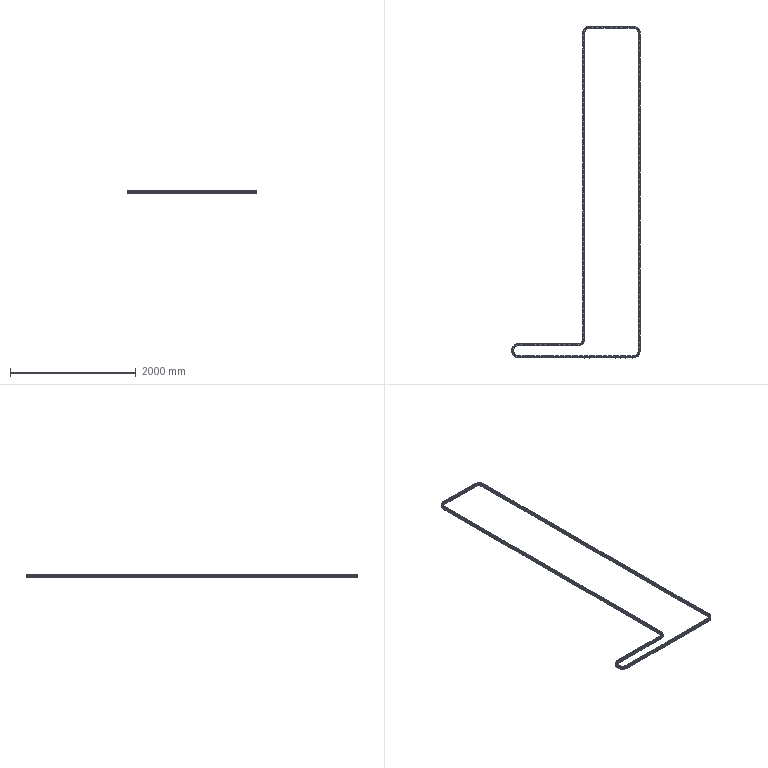Part | STEP file | Outer chain 1XG | 187 solids | 4114 faces | volume 6318542 mm3 | cylinder 3366 | plane 748 | commonest cylinder face diameters 35 x1122 11 x748 22 x748 71.643 x748